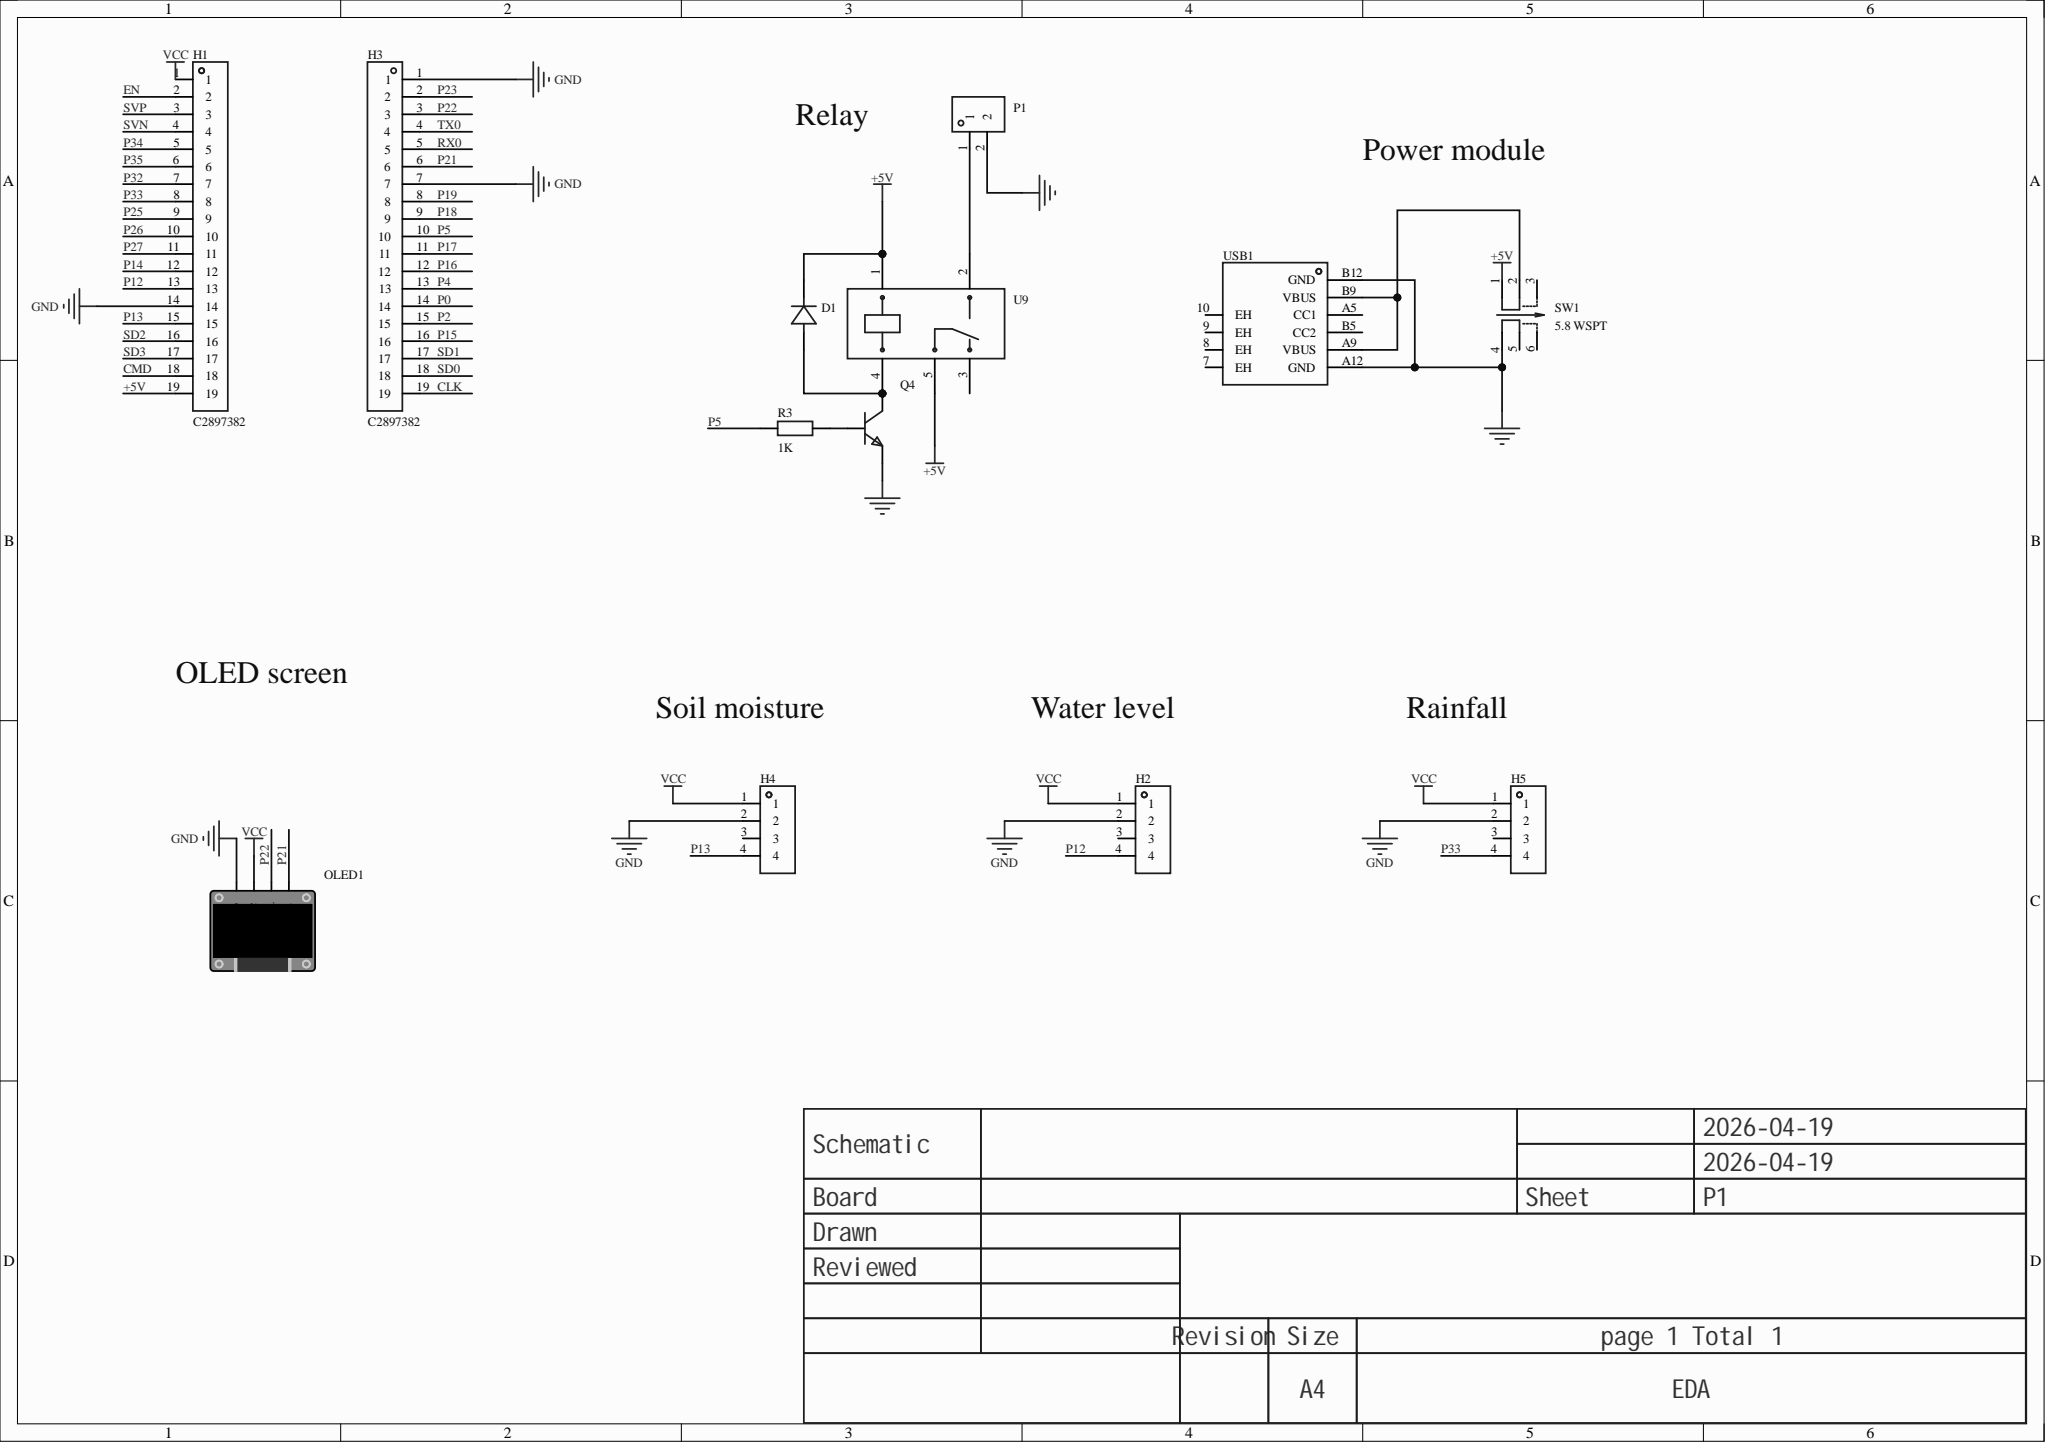Circuit board | Altium Designer | 13 parts | 13 nets
Bill of materials:
Comment,Description,Designator,Footprint,LibRef,Quantity
"","","D1","DO_1N4007","D_1N4007A","1"
"C2897382","","H1, H3","HDR-TH_19P-P2.54-V-F","HDR-F_2.54_1x19P","2"
"","","H2, H4, H5","HDR-TH_4P-P2.54-V-F","HDR-F_2.54_1x4P","3"
"","","OLED1","0.96OLED_4P","0.96OLED模块_4P","1"
"WAFER-XH254Z-2A","Pin structure: 1x2P; Pitch: 2.54mm; Mounting: through-hole; Reference series: XH; Total pins: 2P; Rows: 1; Pins per row: 2; Rated current: 3A; Operating temperature range: -25℃~+85℃;","P1","CONN-TH_2P-P2.50_XH-2A_3045048","WAFER-XH254Z-2A","1"
"","","Q4","S8050_TO_92","S8050_TO_NPN","1"
"1K","","R3","Res_1/8W","Res_AXIAL-1/8W","1"
"5.8 WSPT","Circuit structure: DPDT; Self-lock/no-lock: no lock; Mounting: through-hole; Contact current: 100mA; Rated voltage (AC): -; Rated voltage (DC): 30V; With lamp: no; Actuating force: 1.8N; Mechanical life: 5 thousand cycles;","SW1","SW-TH_6P-L5.8-W5.8-P2.00-LS4.5-TL_K8-5851E-L1","5.8 WSPT","1"
"SRD-12VDC-SL-C","Coil voltage: 12V; Contact form: one changeover group: 1C (SPDT); Contact rating (resistive load): -; Max switching voltage: 250V@AC; Max switching current: 15A;","U9","RELAY-TH_SRD-XXVDC-XL-C","SRD-12VDC-SL-C","1"
"","","USB1","USB_ TYPE-C-6P","USB_ Type-C-6P","1"
Netlist (Protel format):
[
D1
DO_1N4007




]
[
H1
HDR-TH_19P-P2.54-V-F
C2897382



]
[
H2
HDR-TH_4P-P2.54-V-F




]
[
H3
HDR-TH_19P-P2.54-V-F
C2897382



]
[
H4
HDR-TH_4P-P2.54-V-F




]
[
H5
HDR-TH_4P-P2.54-V-F




]
[
OLED1
0.96OLED_4P




]
[
P1
CONN-TH_2P-P2.50_XH-2A_3045048
WAFER-XH254Z-2A



]
[
Q4
S8050_TO_92




]
[
R3
Res_1/8W
1K



]
[
SW1
SW-TH_6P-L5.8-W5.8-P2.00-LS4.5-TL_K8-5851E-L1
5.8 WSPT



]
[
U9
RELAY-TH_SRD-XXVDC-XL-C
SRD-12VDC-SL-C



]
[
USB1
USB_ TYPE-C-6P




]
(
VCC
H1-1
H2-1
H4-1
H5-1
OLED1-2
)
(
P33
H1-8
H5-4
)
(
P22
H3-3
OLED1-3
)
(
P21
H3-6
OLED1-4
)
(
P13
H1-15
H4-4
)
(
P12
H1-13
H2-4
)
(
P5
H3-10
R3-1
)
(
NetSW1_2
SW1-2
USB1-A9
USB1-B9
)
(
NetQ4_2
Q4-2
R3-2
)
(
NetP1_1
P1-1
U9-2
)
(
NetD1_2
D1-2
Q4-3
U9-4
)
(
GND
H1-14
H2-2
H3-1
H3-7
H4-2
H5-2
OLED1-1
P1-2
Q4-1
SW1-4
USB1-A12
USB1-B12
)
(
+5V
D1-1
H1-19
SW1-1
U9-1
U9-5
)